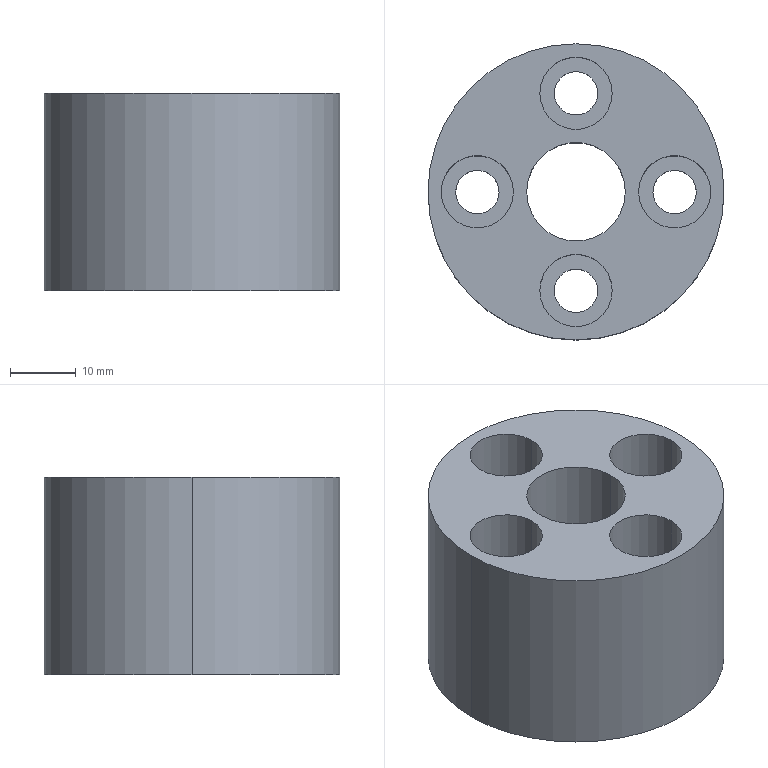Part | STEP file | Locating Pin Seat | 1 solid | 29 faces | box 45 x 45 x 30 mm | volume 32214 mm3 | cylinder 22 | plane 7 | commonest cylinder face diameters 6.6 x8 11 x8 15 x2 20.5 x2 45 x2